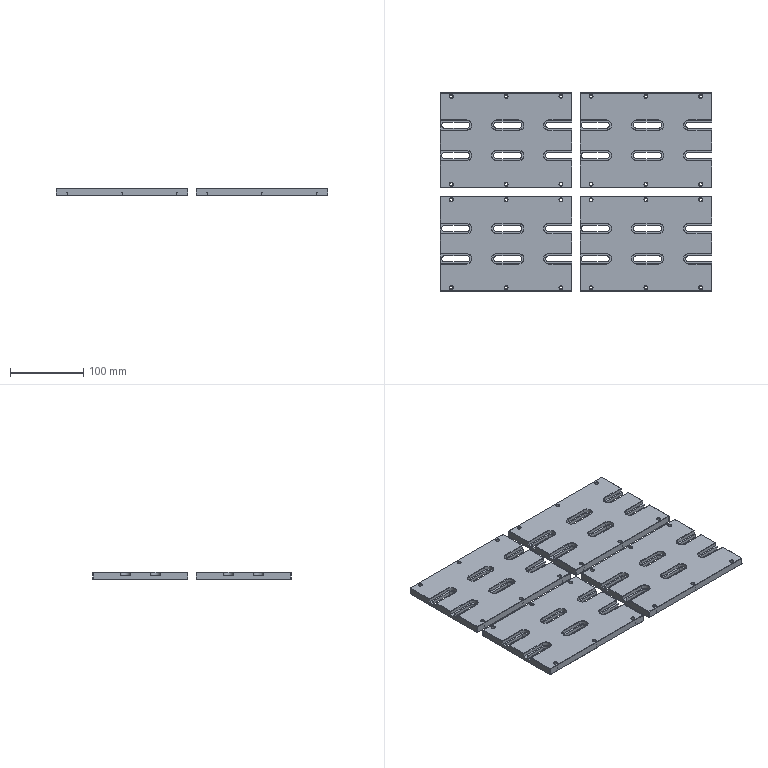NC program | NX | posted with a generic post | part box 371 x 271 x 10 mm
Whole program:
N10 G17 G21 G94 G90
(ZLEVEL_PROFILE_1_COPY_1_COPY_COPY , TOOL : D4A45)
N12 T02 M6
N14 G54
N16 G17 G0 G90 X13.526 Y23.647 S9500 M3
N18 G43 Z30. H2
N20 Z0.
N22 G94 G1 Z-1. F1000.
N24 X13.125 Y24.341
N26 G3 X12.779 Y24.541 R0.4
N28 G1 X-17.22
N30 G3 X-21.011 Y20.75 R3.791
N32 X-17.219 Y16.959 R3.791
N34 G1 X12.78
N36 G3 X16.571 Y20.75 R3.791
N38 X12.779 Y24.541 R3.791
N40 X12.432 Y24.341 R0.4
N42 G1 X12.086 Y23.741
N44 Z0.
N46 G0 Z30.
N48 X-74.248 Y62.688
N50 Z0.
N52 G1 Z-1.
N54 X-74.654 Y63.391
N56 G3 X-75. Y63.591 R0.4
N58 X-78.591 Y60. R3.591
N60 X-75. Y63.591 R-3.591
N62 X-75.346 Y63.391 R0.4
N64 G1 X-75.752 Y62.688
N66 Z0.
N68 G0 Z30.
N70 X-0.752 Y-62.688
N72 Z0.
N74 G1 Z-1.
N76 X-0.346 Y-63.391
N78 G3 X0. Y-63.591 R0.4
N80 G1 X0.006
N82 G3 X3.591 Y-59.994 R3.591
N84 X0. Y-63.591 R-3.591
N86 X0.346 Y-63.391 R0.4
N88 G1 X0.752 Y-62.688
N90 Z0.
N92 G0 Z30.
N94 X53.229 Y-23.646
N96 Z0.
N98 G1 Z-1.
N100 X53.631 Y-24.341
N102 G3 X53.977 Y-24.541 R0.4
N104 G1 X83.98
N106 G3 X87.771 Y-20.75 R3.791
N108 X83.975 Y-16.959 R3.791
N110 G1 X53.98
N112 G3 X50.189 Y-20.75 R3.791
N114 X53.977 Y-24.541 R3.791
N116 X54.324 Y-24.342 R0.4
N118 G1 X54.671 Y-23.741
N120 Z0.
N122 G0 Z30.
N124 X53.229 Y17.854
N126 Z0.
N128 G1 Z-1.
N130 X53.631 Y17.159
N132 G3 X53.977 Y16.959 R0.4
N134 G1 X83.98
N136 G3 X87.771 Y20.75 R3.791
N138 X83.975 Y24.541 R3.791
N140 G1 X53.98
N142 G3 X50.189 Y20.75 R3.791
N144 X53.977 Y16.959 R3.791
N146 X54.324 Y17.158 R0.4
N148 G1 X54.671 Y17.759
N150 Z0.
N152 G0 Z30.
N154 X-75.752 Y-62.688
N156 Z0.
N158 G1 Z-1.
N160 X-75.346 Y-63.391
N162 G3 X-75. Y-63.591 R0.4
N164 G1 X-74.995
N166 G3 X-71.409 Y-59.995 R3.591
N168 X-75. Y-63.591 R-3.591
N170 X-74.654 Y-63.391 R0.4
N172 G1 X-74.248 Y-62.688
N174 Z0.
N176 G0 Z30.
N178 X-17.967 Y-23.647
N180 Z0.
N182 G1 Z-1.
N184 X-17.566 Y-24.341
N186 G3 X-17.219 Y-24.541 R0.4
N188 G1 X12.78
N190 G3 X16.571 Y-20.75 R3.791
N192 X12.779 Y-16.959 R3.791
N194 G1 X-17.22
N196 G3 X-21.011 Y-20.75 R3.791
N198 X-17.219 Y-24.541 R3.791
N200 X-16.873 Y-24.341 R0.4
N202 G1 X-16.527 Y-23.741
N204 Z0.
N206 G0 Z30.
N208 X74.248 Y-62.688
N210 Z0.
N212 G1 Z-1.
N214 X74.654 Y-63.391
N216 G3 X75. Y-63.591 R0.4
N218 X78.591 Y-60. R3.591
N220 X75. Y-63.591 R-3.591
N222 X75.346 Y-63.391 R0.4
N224 G1 X75.752 Y-62.688
N226 Z0.
N228 G0 Z30.
N230 Y62.688
N232 Z0.
N234 G1 Z-1.
N236 X75.346 Y63.391
N238 G3 X75. Y63.591 R0.4
N240 G1 X74.995
N242 G3 X71.409 Y59.995 R3.591
N244 X75. Y63.591 R-3.591
N246 X74.654 Y63.391 R0.4
N248 G1 X74.248 Y62.688
N250 Z0.
N252 G0 Z30.
N254 X0.752
N256 Z0.
N258 G1 Z-1.
N260 X0.346 Y63.391
N262 G3 X0. Y63.591 R0.4
N264 G1 X-0.006
N266 G3 X-3.591 Y59.994 R3.591
N268 X0. Y63.591 R-3.591
N270 X-0.346 Y63.391 R0.4
N272 G1 X-0.752 Y62.688
N274 Z0.
N276 G0 Z30.
N278 X-90.126 Y66.143
N280 Z0.
N282 G1 Z-1.
N284 X-89.846 Y65.659
N286 G3 X-89.5 Y65.459 R0.4
N288 G1 X89.5
N290 G2 X90.459 Y64.5 R0.959
N292 G1 Y-64.5
N294 G2 X89.5 Y-65.459 R0.959
N296 G1 X-89.5
N298 G2 X-90.459 Y-64.5 R0.959
N300 G1 Y-25.
N302 G2 X-89.607 Y-24.352 R0.676
N304 G3 X-88.409 Y-24.541 R3.874
N306 G1 X-58.42
N308 G3 X-54.629 Y-20.75 R3.791
N310 X-58.418 Y-16.959 R3.791
N312 G1 X-88.409
N314 G3 X-89.607 Y-17.148 R3.864
N316 G2 X-90.459 Y-16.501 R0.674
N318 G1 Y16.482
N320 G2 X-89.607 Y17.147 R0.673
N322 G3 X-88.409 Y16.959 R4.012
N324 G1 X-58.42
N326 G3 X-54.629 Y20.75 R3.791
N328 X-58.418 Y24.541 R3.791
N330 G1 X-88.409
N332 G3 X-89.607 Y24.352 R3.982
N334 G2 X-90.459 Y25. R0.676
N336 G1 Y64.5
N338 G2 X-89.5 Y65.459 R0.959
N340 G3 X-89.154 Y65.659 R0.4
N342 G1 X-88.807 Y66.259
N344 Z0.
N346 G0 Z30.
N348 M5
N350 M2